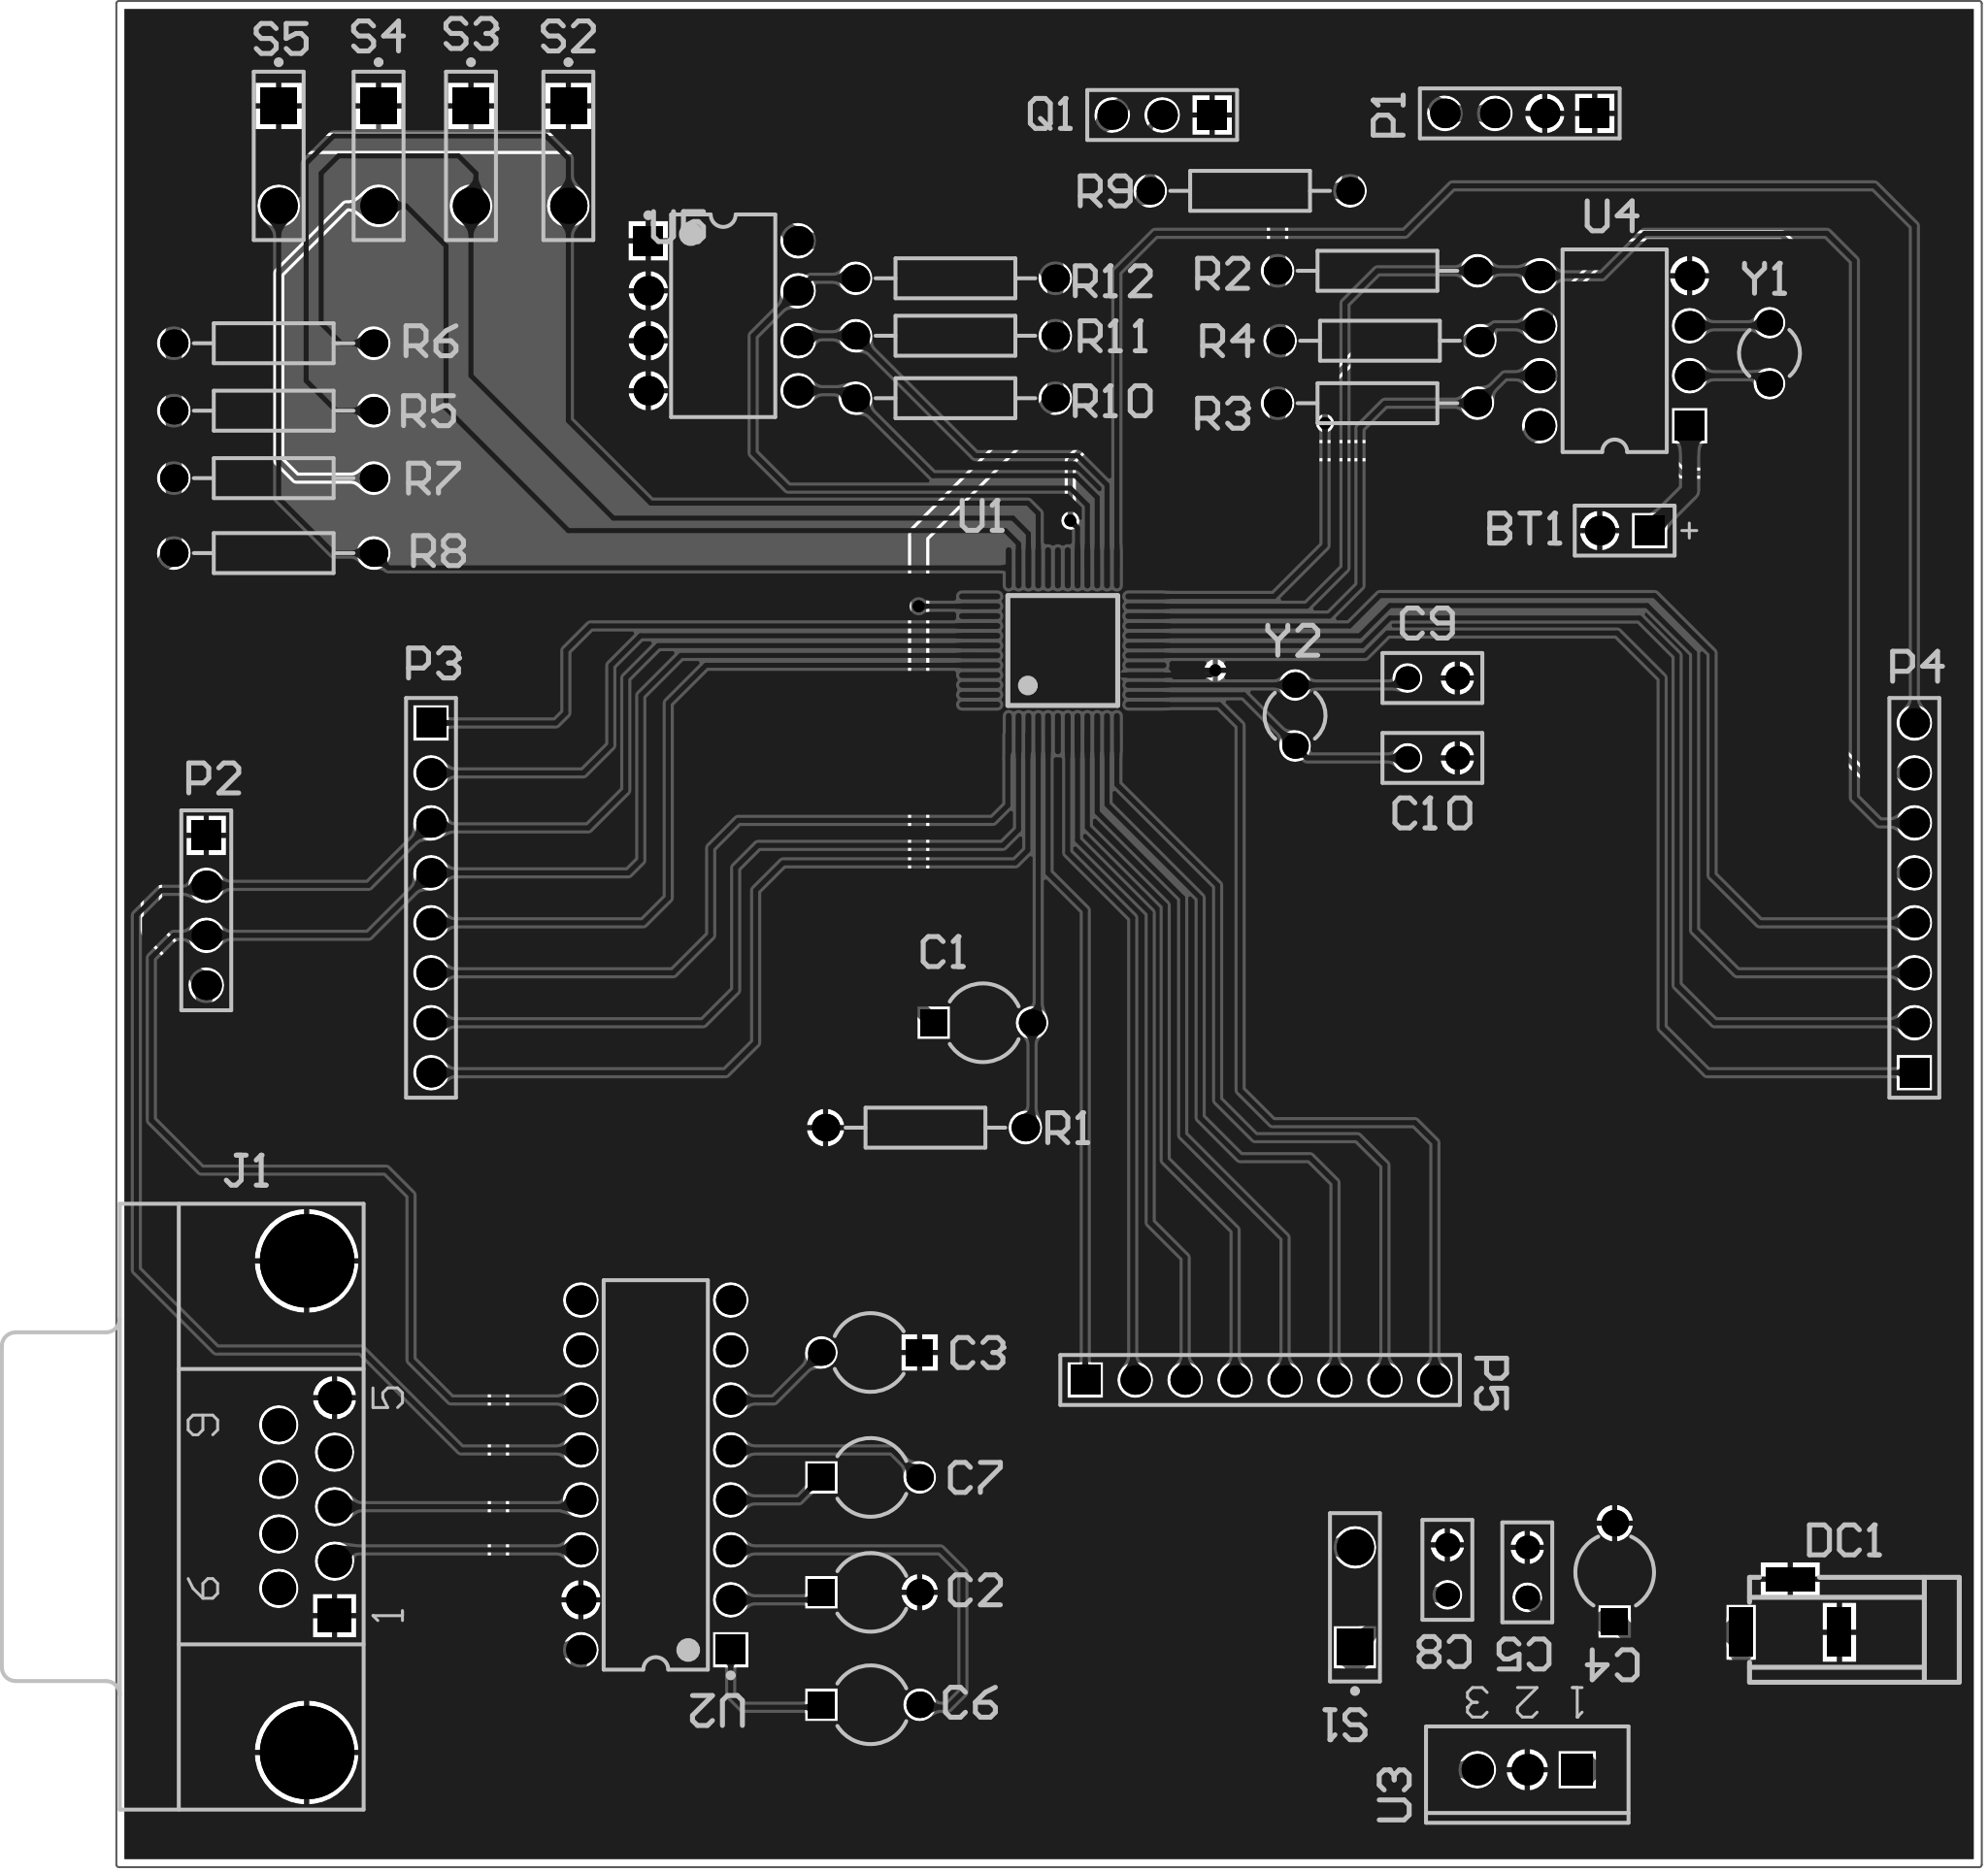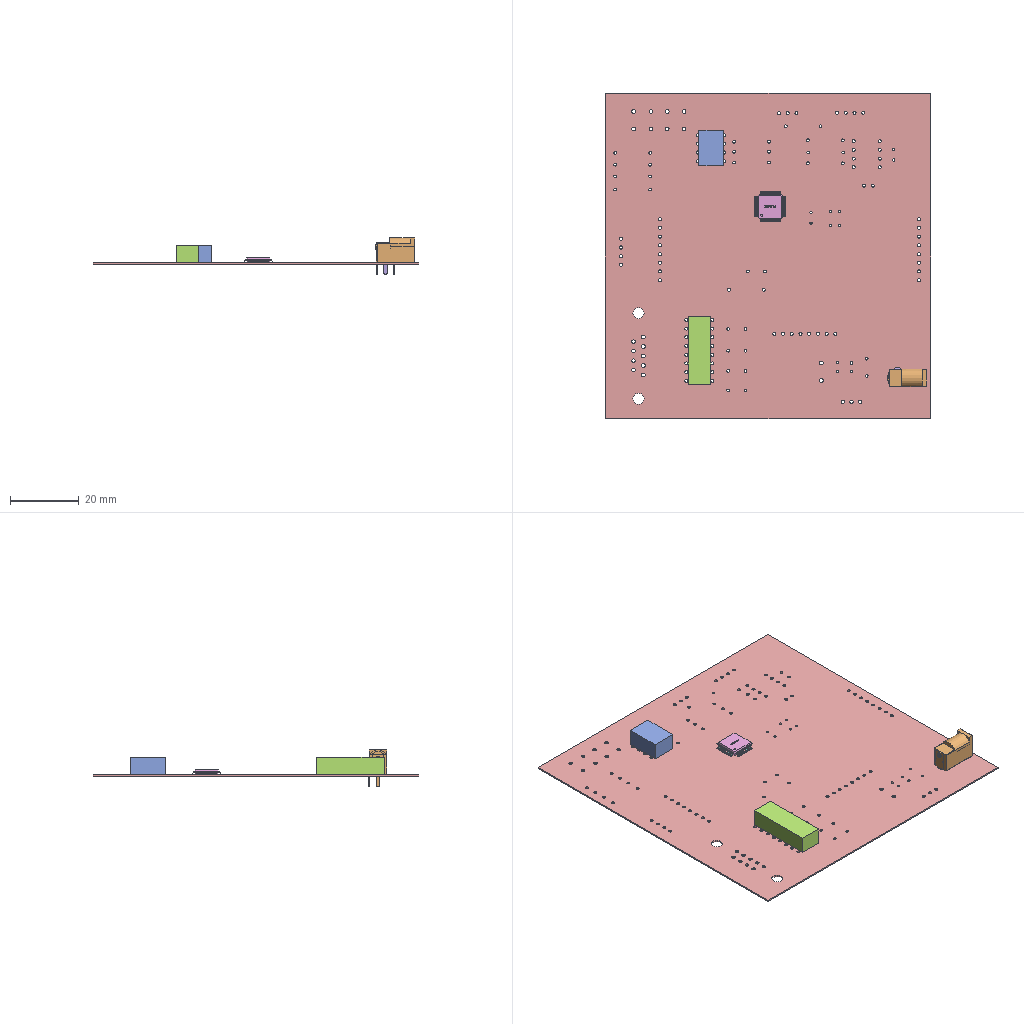Circuit board layout | Altium Designer | box 94.9 x 94.9 x 10.7 mm
Layer stack:
# Altium Designer layer stack of  (unit mm; dielectric type: 0 none, 1 core, 2 prepreg, 3 surface material)
index,name,kind,layer,copper_thickness_mm,dielectric_type,dielectric_thickness_mm,dielectric_material,dielectric_constant
0,Top Paste,other,,,,,,
1,Top Overlay,other,,,,,,
2,Top Solder,dielectric,,,3,0.0102,Solder Resist,3.5
3,Top Layer,copper,Top Layer,0.0356,,,,
4,Dielectric 1,dielectric,,,0,0.32,FR-4,4.8
5,Bottom Layer,copper,Bottom Layer,0.0356,,,,
6,Bottom Solder,dielectric,,,3,0.0102,Solder Resist,3.5
7,Bottom Overlay,other,,,,,,
8,Bottom Paste,other,,,,,,
# drill layer pairs: low layer,high layer
drill_pair,Top Layer,Bottom Layer
Part placement:
Designator,Comment,Layer,Footprint,Center-X(mm),Center-Y(mm),Rotation
Y2,XTAL,TopLayer,R38,112.522,88.265,0
Y1,XTAL,TopLayer,R38,136.652,106.68,180
U5,AT24C01,TopLayer,DIP-8,83.439,108.585,360
U4,DS1302,TopLayer,DIP8,128.778,106.807,90
U3,MC7805BT,TopLayer,221A-04,124.333,34.671,180
U2,MAX232ACPE,TopLayer,PE16A,80.01,49.657,180
U1,STC32C5A60S2,TopLayer,LQFP48_7X7,100.711,91.554,0
S5,SW-PB,TopLayer,SPST-2,60.833,116.713,270
S4,SW-PB,TopLayer,SPST-2,65.913,116.713,270
S3,SW-PB,TopLayer,SPST-2,70.612,116.713,270
S2,SW-PB,TopLayer,SPST-2,75.565,116.713,270
S1,SW-SPST,TopLayer,SPST-2,115.57,43.434,90
R12,Res2,TopLayer,AXIAL-0.4,95.25,110.49,180
R11,Res2,TopLayer,AXIAL-0.4,95.25,107.569,180
R10,Res2,TopLayer,AXIAL-0.4,95.25,104.394,180
R9,Res2,TopLayer,AXIAL-0.4,110.236,114.935,180
R8,Res2,TopLayer,AXIAL-0.4,60.579,96.52,180
R7,Res2,TopLayer,AXIAL-0.4,60.579,100.33,180
R6,Res2,TopLayer,AXIAL-0.4,60.579,107.188,180
R5,Res2,TopLayer,AXIAL-0.4,60.579,103.759,180
R4,Res2,TopLayer,AXIAL-0.4,116.84,107.315,360
R3,Res2,TopLayer,AXIAL-0.4,116.713,104.14,180
R2,Res2,TopLayer,AXIAL-0.4,116.713,110.871,180
R1,Res2,TopLayer,AXIAL-0.4,93.726,67.31,360
Q1,DS18B20,TopLayer,HDR1X3,105.764,118.791,180
P5,Header 8,TopLayer,HDR1X8,110.744,54.483,360
P4,Header 8,TopLayer,HDR1X8,144.018,78.994,90
P3,Header 8,TopLayer,HDR1X8,68.58,78.994,270
P2,Header 4,TopLayer,HDR1X4,57.15,78.359,270
P1,Header 4,TopLayer,HDR1X4,123.952,118.872,180
J1,D Connector 9,TopLayer,DSUB1.385-2H9,62.253,48.042,90
DC1,DC_Socket,TopLayer,DC-002,137.708,43.006,360
C10,Cap,TopLayer,RAD-0.1,119.507,86.106,180
C9,Cap,TopLayer,RAD-0.1,119.507,90.17,180
C8,Cap,TopLayer,RAD-0.1,120.269,44.831,270
C7,Cap2,TopLayer,CAPR5-4X5,90.932,49.53,360
C6,Cap2,TopLayer,CAPR5-4X5,90.932,37.973,0
C5,Cap,TopLayer,RAD-0.1,124.333,44.704,270
C4,Cap2,TopLayer,CAPR5-4X5,128.778,44.704,90
C3,Cap2,TopLayer,CAPR5-4X5,90.932,55.88,180
C2,Cap2,TopLayer,CAPR5-4X5,90.932,43.688,0
C1,Cap2,TopLayer,CAPR5-4X5,96.647,72.644,0
BT1,Battery,TopLayer,BAT-2,129.286,97.663,180
Pad and via stacks:
# Altium Designer via and pad stacks of  (unit mm). Each distinct definition once, with the count of objects using it.
# via: kind,start_layer,end_layer,hole_mm,diameter_mm,mode(0 simple;1 top-mid-bottom;2 full stack),diameter_per_layer,count,example_net
# pad: kind,layer,hole_mm,hole_type(0 round;1 square;2 slot),plating,top_size,top_shape(1 round;2 rect;3 octagon;9 rounded rect),mid_size,bottom_size,mode,footprint,size_per_layer,count,example
pad,Multi-Layer,0.9,0,plated,1.5x1.5,1,1.5x1.5,1.5x1.5,0,BAT-2,,1,BT1.2
pad,Multi-Layer,0.9,0,plated,1.5x1.5,2,1.5x1.5,1.5x1.5,0,BAT-2,,1,BT1.1
pad,Multi-Layer,0.8,0,plated,1.35x1.35,1,1.35x1.35,1.35x1.35,0,CAPR5-4X5,,6,C7.2
pad,Multi-Layer,0.8,0,plated,1.35x1.35,2,1.35x1.35,1.35x1.35,0,CAPR5-4X5,,6,C7.1
pad,Multi-Layer,0.7,0,plated,1.2x1.2,1,1.2x1.2,1.2x1.2,0,RAD-0.1,,8,C10.1
pad,Multi-Layer,0.6,2,plated,2.5x1.2,2,2.5x1.2,2.5x1.2,0,DC-002,,3,DC1.3
pad,Multi-Layer,3.26,0,plated,4.76x4.76,1,4.76x4.76,4.76x4.76,0,DSUB1.385-2H9,,2,J1.11
pad,Multi-Layer,1.09,0,plated,1.69x1.69,2,1.69x1.69,1.69x1.69,0,DSUB1.385-2H9,,1,J1.1
pad,Multi-Layer,1.09,0,plated,1.69x1.69,1,1.69x1.69,1.69x1.69,0,DSUB1.385-2H9,,8,J1.6
pad,Multi-Layer,0.9,0,plated,1.5x1.5,1,1.5x1.5,1.5x1.5,0,HDR1X4,,6,P2.4
pad,Multi-Layer,0.9,0,plated,1.5x1.5,2,1.5x1.5,1.5x1.5,0,HDR1X4,,2,P2.1
pad,Multi-Layer,0.9,0,plated,1.5x1.5,2,1.5x1.5,1.5x1.5,0,HDR1X8,,3,P5.1
pad,Multi-Layer,0.9,0,plated,1.5x1.5,1,1.5x1.5,1.5x1.5,0,HDR1X8,,21,P5.2
pad,Multi-Layer,0.9,0,plated,1.5x1.5,2,1.5x1.5,1.5x1.5,0,HDR1X3,,1,Q1.1
pad,Multi-Layer,0.9,0,plated,1.5x1.5,1,1.5x1.5,1.5x1.5,0,HDR1X3,,2,Q1.2
pad,Multi-Layer,0.85,0,plated,1.4x1.4,1,1.4x1.4,1.4x1.4,0,AXIAL-0.4,,24,R12.1
pad,Multi-Layer,1.1,0,plated,1.85x1.85,2,1.85x1.85,1.85x1.85,0,SPST-2,,5,S5.1
pad,Multi-Layer,1.1,0,plated,1.85x1.85,1,1.85x1.85,1.85x1.85,0,SPST-2,,5,S5.2
pad,Multi-Layer,0.9,0,plated,1.5x1.5,1,1.5x1.5,1.5x1.5,0,PE16A,,15,U2.9
pad,Multi-Layer,0.9,0,plated,1.5x1.5,2,1.5x1.5,1.5x1.5,0,PE16A,,1,U2.1
pad,Multi-Layer,1,0,plated,1.6x1.6,2,1.6x1.6,1.6x1.6,0,221A-04,,1,U3.1
pad,Multi-Layer,1,0,plated,1.6x1.6,1,1.6x1.6,1.6x1.6,0,221A-04,,2,U3.2
pad,Multi-Layer,0.9,0,plated,1.5x1.5,1,1.5x1.5,1.5x1.5,0,DIP8,,7,U4.5
pad,Multi-Layer,0.9,0,plated,1.5x1.5,2,1.5x1.5,1.5x1.5,0,DIP8,,1,U4.1
pad,Multi-Layer,0.9,0,plated,1.5x1.5,2,1.5x1.5,1.5x1.5,0,DIP-8,,1,U5.1
pad,Multi-Layer,0.9,0,plated,1.5x1.5,1,1.5x1.5,1.5x1.5,0,DIP-8,,7,U5.2
pad,Multi-Layer,0.7,0,plated,1.3x1.3,1,1.3x1.3,1.3x1.3,0,R38,,4,Y2.1
pad,Top Layer,0,0,plated,0.3x2.1,1,0.3x2.1,0.3x2.1,0,LQFP48 7X7,,48,U1.48
via,Top Layer,Bottom Layer,0.3048,0.6096,0,,4,VCC
Copper pours:
name,layer,net,type(0 solid;1 hatched;2 none)
D,Bottom Layer,GND,0
D,Top Layer,GND,0
Design rules, without the lines most boards share:
# Altium Designer design rules of  (exported by Altium Designer, unit mm)
# columns: name | kind | enabled | priority | scope1 | scope2 | descriptor | typed fields (field=value)
SilkToSilkClearance | 55 | enabled | 1 | All | All | Silk to Silk (Clearance=0mil) (All),(All) |
SilkToSolderMaskClearance | 54 | enabled | 1 | IsPad | All | Silk To Solder Mask (Clearance=0mil) (IsPad),(All) |
MinimumSolderMaskSliver | 53 | enabled | 1 | All | All | Minimum Solder Mask Sliver (Gap=0mil) (All),(All) |
HoleToHoleClearance | 52 | enabled | 1 | All | All | Hole To Hole Clearance (Gap=10mil) (All),(All) | gap=0.254
DiffPairsRouting | 51 | enabled | 1 | All | All | Differential Pairs Uncoupled Length using the Gap Constraints (Min=10mil) (Max=10mil) (Prefered=10mil)  and Width Constraints (Min=15mil) (Max=15mil) (Prefered=15mil) (All) |
HoleSize | 42 | enabled | 1 | All | All | Hole Size Constraint (Min=1mil) (Max=99999mil) (All) |
SolderMaskExpansion | 13 | enabled | 1 | All | All | Solder Mask Expansion (Expansion =4mil) (All) | expansion=0.1016
PasteMaskExpansion | 14 | enabled | 1 | All | All | Paste Mask Expansion (Expansion =0mil) (All) | expansion=0
RoutingVias | 11 | enabled | 1 | All | All | Routing Via (MinHoleWidth=28mil) (MaxHoleWidth=28mil) (PreferredHoleWidth=28mil) (MinWidth=50mil) (MaxWidth=50mil) (PreferedWidth=50mil) (All) | via_min_hole=0.7112 via_max_hole=0.7112 via_preferred_diameter=1.27 via_preferred_hole=0.7112
Width | 2 | enabled | 1 | All | All | Width Constraint (Min=10mil) (Max=30mil) (Preferred=10mil) (All) |
PolygonConnect | 20 | enabled | 1 | All | All | Polygon Connect Rule(Relief Connect )(Conductor Width=10mil) (Relief Angle=90 Angle) (Entries=4) (Air Gap Width=10mil) (All),(All) | connect_style(0=relief,1=direct,2=none)=0 relief_conductor_width=0.254 relief_entries=4
PlaneConnect | 6 | enabled | 1 | All | All | Power Plane Connect Rule(Relief Connect )(Expansion=20mil) (Conductor Width=10mil) (Air Gap=10mil) (Entries=4) (All) | relief_conductor_width=0.254 relief_entries=4 relief_expansion=0.508
Clearance | 0 | enabled | 1 | All | All | Clearance Constraint (Gap=6mil) (All),(All) | gap=0.1524
Classes set for this board:
# Altium Designer classes of  (member kind: 0 net, 1 component, 2 from-to, 3 pad, 4 layer, 5 differential pair, 6 design channel, 7 polygon, 8 structure, 9 xSignal)
# columns: class name | member kind | superclass | members
Sheet1 | 1 | no | BT1; C1; C2; C3; C4; C5; C6; C7; C8; C9; C10; DC1; J1; P1; P2; P3; P4; P5; Q1; R1; R2; R3; R4; R5; R6; R7; R8; R9; R10; R11; R12; S1; S2; S3; S4; S5; U1; U2; U3; U4; U5; Y1; Y2;